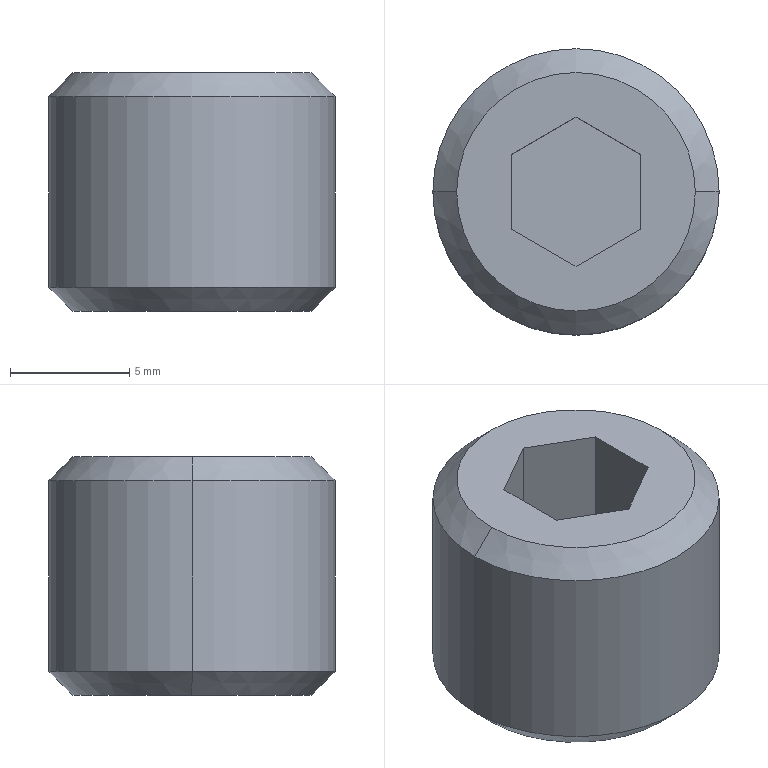Part | SolidWorks | features Chamfer 1, Extrusion 1, ICE 1 | 1 solid | 15 faces | box 12 x 12 x 10 mm | volume 968.16 mm3 | plane 9 | cone 4 | cylinder 2 | commonest cylinder face diameters 12 x2
STEP:
#1=CARTESIAN_POINT('',(-5.,0.,0.));
#2=VERTEX_POINT('',#1);
#3=CARTESIAN_POINT('',(5.,0.,0.));
#4=VERTEX_POINT('',#3);
#5=CARTESIAN_POINT('',(0.,0.,0.));
#6=DIRECTION('',(0.,0.,-1.));
#7=DIRECTION('',(1.,0.,0.));
#8=AXIS2_PLACEMENT_3D('',#5,#6,#7);
#9=CIRCLE('',#8,5.);
#10=EDGE_CURVE('',#2,#4,#9,.T.);
#11=ORIENTED_EDGE('',*,*,#10,.F.);
#12=CARTESIAN_POINT('',(-6.,0.,1.));
#13=VERTEX_POINT('',#12);
#14=CARTESIAN_POINT('',(-6.,0.,1.));
#15=DIRECTION('',(-0.7071,0.,0.7071));
#16=VECTOR('',#15,1000.);
#17=LINE('',#14,#16);
#18=EDGE_CURVE('',#2,#13,#17,.T.);
#19=ORIENTED_EDGE('',*,*,#18,.T.);
#20=CARTESIAN_POINT('',(6.,0.,1.));
#21=VERTEX_POINT('',#20);
#22=CARTESIAN_POINT('',(0.,0.,1.));
#23=DIRECTION('',(0.,0.,1.));
#24=DIRECTION('',(1.,0.,0.));
#25=AXIS2_PLACEMENT_3D('',#22,#23,#24);
#26=CIRCLE('',#25,6.);
#27=EDGE_CURVE('',#21,#13,#26,.T.);
#28=ORIENTED_EDGE('',*,*,#27,.F.);
#29=CARTESIAN_POINT('',(6.,0.,1.));
#30=DIRECTION('',(0.7071,0.,0.7071));
#31=VECTOR('',#30,1000.);
#32=LINE('',#29,#31);
#33=EDGE_CURVE('',#4,#21,#32,.T.);
#34=ORIENTED_EDGE('',*,*,#33,.F.);
#35=EDGE_LOOP('',(#11,#19,#28,#34));
#36=FACE_OUTER_BOUND('',#35,.T.);
#37=CARTESIAN_POINT('',(0.,0.,1.));
#38=DIRECTION('',(0.,0.,1.));
#39=DIRECTION('',(1.,0.,0.));
#40=AXIS2_PLACEMENT_3D('',#37,#38,#39);
#41=CONICAL_SURFACE('',#40,6.,0.7854);
#42=ADVANCED_FACE('',(#36),#41,.T.);
#43=CARTESIAN_POINT('',(5.,0.,10.));
#44=VERTEX_POINT('',#43);
#45=CARTESIAN_POINT('',(-5.,0.,10.));
#46=VERTEX_POINT('',#45);
#47=CARTESIAN_POINT('',(0.,0.,10.));
#48=DIRECTION('',(0.,0.,1.));
#49=DIRECTION('',(1.,0.,0.));
#50=AXIS2_PLACEMENT_3D('',#47,#48,#49);
#51=CIRCLE('',#50,5.);
#52=EDGE_CURVE('',#44,#46,#51,.T.);
#53=ORIENTED_EDGE('',*,*,#52,.F.);
#54=CARTESIAN_POINT('',(6.,0.,9.));
#55=VERTEX_POINT('',#54);
#56=CARTESIAN_POINT('',(5.,0.,10.));
#57=DIRECTION('',(0.7071,0.,-0.7071));
#58=VECTOR('',#57,1000.);
#59=LINE('',#56,#58);
#60=EDGE_CURVE('',#44,#55,#59,.T.);
#61=ORIENTED_EDGE('',*,*,#60,.T.);
#62=CARTESIAN_POINT('',(-6.,0.,9.));
#63=VERTEX_POINT('',#62);
#64=CARTESIAN_POINT('',(0.,0.,9.));
#65=DIRECTION('',(0.,0.,-1.));
#66=DIRECTION('',(1.,0.,0.));
#67=AXIS2_PLACEMENT_3D('',#64,#65,#66);
#68=CIRCLE('',#67,6.);
#69=EDGE_CURVE('',#63,#55,#68,.T.);
#70=ORIENTED_EDGE('',*,*,#69,.F.);
#71=CARTESIAN_POINT('',(-5.,0.,10.));
#72=DIRECTION('',(-0.7071,0.,-0.7071));
#73=VECTOR('',#72,1000.);
#74=LINE('',#71,#73);
#75=EDGE_CURVE('',#46,#63,#74,.T.);
#76=ORIENTED_EDGE('',*,*,#75,.F.);
#77=EDGE_LOOP('',(#53,#61,#70,#76));
#78=FACE_OUTER_BOUND('',#77,.T.);
#79=CARTESIAN_POINT('',(0.,0.,10.));
#80=DIRECTION('',(0.,0.,-1.));
#81=DIRECTION('',(-1.,0.,0.));
#82=AXIS2_PLACEMENT_3D('',#79,#80,#81);
#83=CONICAL_SURFACE('',#82,5.,0.7854);
#84=ADVANCED_FACE('',(#78),#83,.T.);
#85=ORIENTED_EDGE('',*,*,#69,.T.);
#86=CARTESIAN_POINT('',(6.,0.,10.));
#87=DIRECTION('',(0.,0.,-1.));
#88=VECTOR('',#87,1000.);
#89=LINE('',#86,#88);
#90=EDGE_CURVE('',#55,#21,#89,.T.);
#91=ORIENTED_EDGE('',*,*,#90,.T.);
#92=ORIENTED_EDGE('',*,*,#27,.T.);
#93=CARTESIAN_POINT('',(-6.,0.,10.));
#94=DIRECTION('',(0.,0.,-1.));
#95=VECTOR('',#94,1000.);
#96=LINE('',#93,#95);
#97=EDGE_CURVE('',#63,#13,#96,.T.);
#98=ORIENTED_EDGE('',*,*,#97,.F.);
#99=EDGE_LOOP('',(#85,#91,#92,#98));
#100=FACE_OUTER_BOUND('',#99,.T.);
#101=CARTESIAN_POINT('',(0.,0.,10.));
#102=DIRECTION('',(0.,0.,-1.));
#103=DIRECTION('',(-1.,0.,0.));
#104=AXIS2_PLACEMENT_3D('',#101,#102,#103);
#105=CYLINDRICAL_SURFACE('',#104,6.);
#106=ADVANCED_FACE('',(#100),#105,.T.);
#107=ORIENTED_EDGE('',*,*,#90,.F.);
#108=CARTESIAN_POINT('',(0.,0.,9.));
#109=DIRECTION('',(0.,0.,-1.));
#110=DIRECTION('',(1.,0.,0.));
#111=AXIS2_PLACEMENT_3D('',#108,#109,#110);
#112=CIRCLE('',#111,6.);
#113=EDGE_CURVE('',#55,#63,#112,.T.);
#114=ORIENTED_EDGE('',*,*,#113,.T.);
#115=ORIENTED_EDGE('',*,*,#97,.T.);
#116=CARTESIAN_POINT('',(0.,0.,1.));
#117=DIRECTION('',(0.,0.,1.));
#118=DIRECTION('',(1.,0.,0.));
#119=AXIS2_PLACEMENT_3D('',#116,#117,#118);
#120=CIRCLE('',#119,6.);
#121=EDGE_CURVE('',#13,#21,#120,.T.);
#122=ORIENTED_EDGE('',*,*,#121,.T.);
#123=EDGE_LOOP('',(#107,#114,#115,#122));
#124=FACE_OUTER_BOUND('',#123,.T.);
#125=CARTESIAN_POINT('',(0.,0.,10.));
#126=DIRECTION('',(0.,0.,-1.));
#127=DIRECTION('',(-1.,0.,0.));
#128=AXIS2_PLACEMENT_3D('',#125,#126,#127);
#129=CYLINDRICAL_SURFACE('',#128,6.);
#130=ADVANCED_FACE('',(#124),#129,.T.);
#131=CARTESIAN_POINT('',(0.,0.,10.));
#132=DIRECTION('',(0.,0.,1.));
#133=DIRECTION('',(1.,0.,0.));
#134=AXIS2_PLACEMENT_3D('',#131,#132,#133);
#135=CIRCLE('',#134,5.);
#136=EDGE_CURVE('',#46,#44,#135,.T.);
#137=ORIENTED_EDGE('',*,*,#136,.T.);
#138=ORIENTED_EDGE('',*,*,#52,.T.);
#139=EDGE_LOOP('',(#137,#138));
#140=FACE_OUTER_BOUND('',#139,.T.);
#141=CARTESIAN_POINT('',(2.71,1.565,10.));
#142=VERTEX_POINT('',#141);
#143=CARTESIAN_POINT('',(0.,3.129,10.));
#144=VERTEX_POINT('',#143);
#145=CARTESIAN_POINT('',(2.71,1.565,10.));
#146=DIRECTION('',(-0.866,0.5,0.));
#147=VECTOR('',#146,1000.);
#148=LINE('',#145,#147);
#149=EDGE_CURVE('',#142,#144,#148,.T.);
#150=ORIENTED_EDGE('',*,*,#149,.F.);
#151=CARTESIAN_POINT('',(2.71,-1.565,10.));
#152=VERTEX_POINT('',#151);
#153=CARTESIAN_POINT('',(2.71,-1.565,10.));
#154=DIRECTION('',(0.,1.,0.));
#155=VECTOR('',#154,1000.);
#156=LINE('',#153,#155);
#157=EDGE_CURVE('',#152,#142,#156,.T.);
#158=ORIENTED_EDGE('',*,*,#157,.F.);
#159=CARTESIAN_POINT('',(0.,-3.129,10.));
#160=VERTEX_POINT('',#159);
#161=CARTESIAN_POINT('',(0.,-3.129,10.));
#162=DIRECTION('',(0.866,0.5,0.));
#163=VECTOR('',#162,1000.);
#164=LINE('',#161,#163);
#165=EDGE_CURVE('',#160,#152,#164,.T.);
#166=ORIENTED_EDGE('',*,*,#165,.F.);
#167=CARTESIAN_POINT('',(-2.71,-1.565,10.));
#168=VERTEX_POINT('',#167);
#169=CARTESIAN_POINT('',(-2.71,-1.565,10.));
#170=DIRECTION('',(0.866,-0.5,0.));
#171=VECTOR('',#170,1000.);
#172=LINE('',#169,#171);
#173=EDGE_CURVE('',#168,#160,#172,.T.);
#174=ORIENTED_EDGE('',*,*,#173,.F.);
#175=CARTESIAN_POINT('',(-2.71,1.565,10.));
#176=VERTEX_POINT('',#175);
#177=CARTESIAN_POINT('',(-2.71,1.565,10.));
#178=DIRECTION('',(0.,-1.,0.));
#179=VECTOR('',#178,1000.);
#180=LINE('',#177,#179);
#181=EDGE_CURVE('',#176,#168,#180,.T.);
#182=ORIENTED_EDGE('',*,*,#181,.F.);
#183=CARTESIAN_POINT('',(0.,3.129,10.));
#184=DIRECTION('',(-0.866,-0.5,0.));
#185=VECTOR('',#184,1000.);
#186=LINE('',#183,#185);
#187=EDGE_CURVE('',#144,#176,#186,.T.);
#188=ORIENTED_EDGE('',*,*,#187,.F.);
#189=EDGE_LOOP('',(#150,#158,#166,#174,#182,#188));
#190=FACE_BOUND('',#189,.T.);
#191=CARTESIAN_POINT('',(0.,0.,10.));
#192=DIRECTION('',(0.,0.,1.));
#193=DIRECTION('',(1.,0.,0.));
#194=AXIS2_PLACEMENT_3D('',#191,#192,#193);
#195=PLANE('',#194);
#196=ADVANCED_FACE('',(#140,#190),#195,.T.);
#197=CARTESIAN_POINT('',(0.,0.,0.));
#198=DIRECTION('',(0.,0.,-1.));
#199=DIRECTION('',(1.,0.,0.));
#200=AXIS2_PLACEMENT_3D('',#197,#198,#199);
#201=CIRCLE('',#200,5.);
#202=EDGE_CURVE('',#4,#2,#201,.T.);
#203=ORIENTED_EDGE('',*,*,#202,.T.);
#204=ORIENTED_EDGE('',*,*,#10,.T.);
#205=EDGE_LOOP('',(#203,#204));
#206=FACE_OUTER_BOUND('',#205,.T.);
#207=CARTESIAN_POINT('',(0.,0.,0.));
#208=DIRECTION('',(0.,0.,1.));
#209=DIRECTION('',(1.,0.,0.));
#210=AXIS2_PLACEMENT_3D('',#207,#208,#209);
#211=PLANE('',#210);
#212=ADVANCED_FACE('',(#206),#211,.F.);
#213=ORIENTED_EDGE('',*,*,#149,.T.);
#214=CARTESIAN_POINT('',(0.,3.129,5.));
#215=VERTEX_POINT('',#214);
#216=CARTESIAN_POINT('',(0.,3.129,5.));
#217=DIRECTION('',(0.,0.,1.));
#218=VECTOR('',#217,1000.);
#219=LINE('',#216,#218);
#220=EDGE_CURVE('',#215,#144,#219,.T.);
#221=ORIENTED_EDGE('',*,*,#220,.F.);
#222=CARTESIAN_POINT('',(2.71,1.565,5.));
#223=VERTEX_POINT('',#222);
#224=CARTESIAN_POINT('',(2.71,1.565,5.));
#225=DIRECTION('',(-0.866,0.5,0.));
#226=VECTOR('',#225,1000.);
#227=LINE('',#224,#226);
#228=EDGE_CURVE('',#223,#215,#227,.T.);
#229=ORIENTED_EDGE('',*,*,#228,.F.);
#230=CARTESIAN_POINT('',(2.71,1.565,5.));
#231=DIRECTION('',(0.,0.,1.));
#232=VECTOR('',#231,1000.);
#233=LINE('',#230,#232);
#234=EDGE_CURVE('',#223,#142,#233,.T.);
#235=ORIENTED_EDGE('',*,*,#234,.T.);
#236=EDGE_LOOP('',(#213,#221,#229,#235));
#237=FACE_OUTER_BOUND('',#236,.T.);
#238=CARTESIAN_POINT('',(2.71,1.565,5.));
#239=DIRECTION('',(0.5,0.866,0.));
#240=DIRECTION('',(-0.866,0.5,0.));
#241=AXIS2_PLACEMENT_3D('',#238,#239,#240);
#242=PLANE('',#241);
#243=ADVANCED_FACE('',(#237),#242,.F.);
#244=ORIENTED_EDGE('',*,*,#157,.T.);
#245=ORIENTED_EDGE('',*,*,#234,.F.);
#246=CARTESIAN_POINT('',(2.71,-1.565,5.));
#247=VERTEX_POINT('',#246);
#248=CARTESIAN_POINT('',(2.71,-1.565,5.));
#249=DIRECTION('',(0.,1.,0.));
#250=VECTOR('',#249,1000.);
#251=LINE('',#248,#250);
#252=EDGE_CURVE('',#247,#223,#251,.T.);
#253=ORIENTED_EDGE('',*,*,#252,.F.);
#254=CARTESIAN_POINT('',(2.71,-1.565,5.));
#255=DIRECTION('',(0.,0.,1.));
#256=VECTOR('',#255,1000.);
#257=LINE('',#254,#256);
#258=EDGE_CURVE('',#247,#152,#257,.T.);
#259=ORIENTED_EDGE('',*,*,#258,.T.);
#260=EDGE_LOOP('',(#244,#245,#253,#259));
#261=FACE_OUTER_BOUND('',#260,.T.);
#262=CARTESIAN_POINT('',(2.71,-1.565,5.));
#263=DIRECTION('',(1.,0.,0.));
#264=DIRECTION('',(0.,1.,0.));
#265=AXIS2_PLACEMENT_3D('',#262,#263,#264);
#266=PLANE('',#265);
#267=ADVANCED_FACE('',(#261),#266,.F.);
#268=ORIENTED_EDGE('',*,*,#165,.T.);
#269=ORIENTED_EDGE('',*,*,#258,.F.);
#270=CARTESIAN_POINT('',(0.,-3.129,5.));
#271=VERTEX_POINT('',#270);
#272=CARTESIAN_POINT('',(0.,-3.129,5.));
#273=DIRECTION('',(0.866,0.5,0.));
#274=VECTOR('',#273,1000.);
#275=LINE('',#272,#274);
#276=EDGE_CURVE('',#271,#247,#275,.T.);
#277=ORIENTED_EDGE('',*,*,#276,.F.);
#278=CARTESIAN_POINT('',(0.,-3.129,5.));
#279=DIRECTION('',(0.,0.,1.));
#280=VECTOR('',#279,1000.);
#281=LINE('',#278,#280);
#282=EDGE_CURVE('',#271,#160,#281,.T.);
#283=ORIENTED_EDGE('',*,*,#282,.T.);
#284=EDGE_LOOP('',(#268,#269,#277,#283));
#285=FACE_OUTER_BOUND('',#284,.T.);
#286=CARTESIAN_POINT('',(0.,-3.129,5.));
#287=DIRECTION('',(0.5,-0.866,0.));
#288=DIRECTION('',(0.866,0.5,0.));
#289=AXIS2_PLACEMENT_3D('',#286,#287,#288);
#290=PLANE('',#289);
#291=ADVANCED_FACE('',(#285),#290,.F.);
#292=ORIENTED_EDGE('',*,*,#173,.T.);
#293=ORIENTED_EDGE('',*,*,#282,.F.);
#294=CARTESIAN_POINT('',(-2.71,-1.565,5.));
#295=VERTEX_POINT('',#294);
#296=CARTESIAN_POINT('',(-2.71,-1.565,5.));
#297=DIRECTION('',(0.866,-0.5,0.));
#298=VECTOR('',#297,1000.);
#299=LINE('',#296,#298);
#300=EDGE_CURVE('',#295,#271,#299,.T.);
#301=ORIENTED_EDGE('',*,*,#300,.F.);
#302=CARTESIAN_POINT('',(-2.71,-1.565,5.));
#303=DIRECTION('',(0.,0.,1.));
#304=VECTOR('',#303,1000.);
#305=LINE('',#302,#304);
#306=EDGE_CURVE('',#295,#168,#305,.T.);
#307=ORIENTED_EDGE('',*,*,#306,.T.);
#308=EDGE_LOOP('',(#292,#293,#301,#307));
#309=FACE_OUTER_BOUND('',#308,.T.);
#310=CARTESIAN_POINT('',(-2.71,-1.565,5.));
#311=DIRECTION('',(-0.5,-0.866,0.));
#312=DIRECTION('',(0.866,-0.5,0.));
#313=AXIS2_PLACEMENT_3D('',#310,#311,#312);
#314=PLANE('',#313);
#315=ADVANCED_FACE('',(#309),#314,.F.);
#316=ORIENTED_EDGE('',*,*,#181,.T.);
#317=ORIENTED_EDGE('',*,*,#306,.F.);
#318=CARTESIAN_POINT('',(-2.71,1.565,5.));
#319=VERTEX_POINT('',#318);
#320=CARTESIAN_POINT('',(-2.71,1.565,5.));
#321=DIRECTION('',(0.,-1.,0.));
#322=VECTOR('',#321,1000.);
#323=LINE('',#320,#322);
#324=EDGE_CURVE('',#319,#295,#323,.T.);
#325=ORIENTED_EDGE('',*,*,#324,.F.);
#326=CARTESIAN_POINT('',(-2.71,1.565,5.));
#327=DIRECTION('',(0.,0.,1.));
#328=VECTOR('',#327,1000.);
#329=LINE('',#326,#328);
#330=EDGE_CURVE('',#319,#176,#329,.T.);
#331=ORIENTED_EDGE('',*,*,#330,.T.);
#332=EDGE_LOOP('',(#316,#317,#325,#331));
#333=FACE_OUTER_BOUND('',#332,.T.);
#334=CARTESIAN_POINT('',(-2.71,1.565,5.));
#335=DIRECTION('',(-1.,0.,0.));
#336=DIRECTION('',(0.,-1.,0.));
#337=AXIS2_PLACEMENT_3D('',#334,#335,#336);
#338=PLANE('',#337);
#339=ADVANCED_FACE('',(#333),#338,.F.);
#340=ORIENTED_EDGE('',*,*,#187,.T.);
#341=ORIENTED_EDGE('',*,*,#330,.F.);
#342=CARTESIAN_POINT('',(0.,3.129,5.));
#343=DIRECTION('',(-0.866,-0.5,0.));
#344=VECTOR('',#343,1000.);
#345=LINE('',#342,#344);
#346=EDGE_CURVE('',#215,#319,#345,.T.);
#347=ORIENTED_EDGE('',*,*,#346,.F.);
#348=ORIENTED_EDGE('',*,*,#220,.T.);
#349=EDGE_LOOP('',(#340,#341,#347,#348));
#350=FACE_OUTER_BOUND('',#349,.T.);
#351=CARTESIAN_POINT('',(0.,3.129,5.));
#352=DIRECTION('',(-0.5,0.866,0.));
#353=DIRECTION('',(-0.866,-0.5,0.));
#354=AXIS2_PLACEMENT_3D('',#351,#352,#353);
#355=PLANE('',#354);
#356=ADVANCED_FACE('',(#350),#355,.F.);
#357=ORIENTED_EDGE('',*,*,#228,.T.);
#358=ORIENTED_EDGE('',*,*,#346,.T.);
#359=ORIENTED_EDGE('',*,*,#324,.T.);
#360=ORIENTED_EDGE('',*,*,#300,.T.);
#361=ORIENTED_EDGE('',*,*,#276,.T.);
#362=ORIENTED_EDGE('',*,*,#252,.T.);
#363=EDGE_LOOP('',(#357,#358,#359,#360,#361,#362));
#364=FACE_OUTER_BOUND('',#363,.T.);
#365=CARTESIAN_POINT('',(0.,0.,5.));
#366=DIRECTION('',(0.,0.,1.));
#367=DIRECTION('',(1.,0.,0.));
#368=AXIS2_PLACEMENT_3D('',#365,#366,#367);
#369=PLANE('',#368);
#370=ADVANCED_FACE('',(#364),#369,.T.);
#371=ORIENTED_EDGE('',*,*,#60,.F.);
#372=ORIENTED_EDGE('',*,*,#136,.F.);
#373=ORIENTED_EDGE('',*,*,#75,.T.);
#374=ORIENTED_EDGE('',*,*,#113,.F.);
#375=EDGE_LOOP('',(#371,#372,#373,#374));
#376=FACE_OUTER_BOUND('',#375,.T.);
#377=CARTESIAN_POINT('',(0.,0.,10.));
#378=DIRECTION('',(0.,0.,-1.));
#379=DIRECTION('',(-1.,0.,0.));
#380=AXIS2_PLACEMENT_3D('',#377,#378,#379);
#381=CONICAL_SURFACE('',#380,5.,0.7854);
#382=ADVANCED_FACE('',(#376),#381,.T.);
#383=ORIENTED_EDGE('',*,*,#18,.F.);
#384=ORIENTED_EDGE('',*,*,#202,.F.);
#385=ORIENTED_EDGE('',*,*,#33,.T.);
#386=ORIENTED_EDGE('',*,*,#121,.F.);
#387=EDGE_LOOP('',(#383,#384,#385,#386));
#388=FACE_OUTER_BOUND('',#387,.T.);
#389=CARTESIAN_POINT('',(0.,0.,1.));
#390=DIRECTION('',(0.,0.,1.));
#391=DIRECTION('',(1.,0.,0.));
#392=AXIS2_PLACEMENT_3D('',#389,#390,#391);
#393=CONICAL_SURFACE('',#392,6.,0.7854);
#394=ADVANCED_FACE('',(#388),#393,.T.);
#395=CLOSED_SHELL('',(#42,#84,#106,#130,#196,#212,#243,#267,#291,#315,#339,#356,#370,#382,#394));
#396=MANIFOLD_SOLID_BREP('',#395);
#397=CARTESIAN_POINT('',(0.,0.,0.));
#398=DIRECTION('',(0.,0.,1.));
#399=DIRECTION('',(1.,0.,0.));
#400=AXIS2_PLACEMENT_3D('',#397,#398,#399);
#401=(LENGTH_UNIT()NAMED_UNIT(*)SI_UNIT(.MILLI.,.METRE.));
#402=UNCERTAINTY_MEASURE_WITH_UNIT(LENGTH_MEASURE(0.00001),#401,'','');
#403=(NAMED_UNIT(*)PLANE_ANGLE_UNIT()SI_UNIT($,.RADIAN.));
#404=(NAMED_UNIT(*)SI_UNIT($,.STERADIAN.)SOLID_ANGLE_UNIT());
#405=(GEOMETRIC_REPRESENTATION_CONTEXT(3)GLOBAL_UNCERTAINTY_ASSIGNED_CONTEXT((#402))GLOBAL_UNIT_ASSIGNED_CONTEXT((#401,#403,#404))REPRESENTATION_CONTEXT('',''));
#406=ADVANCED_BREP_SHAPE_REPRESENTATION('',(#396,#400),#405);